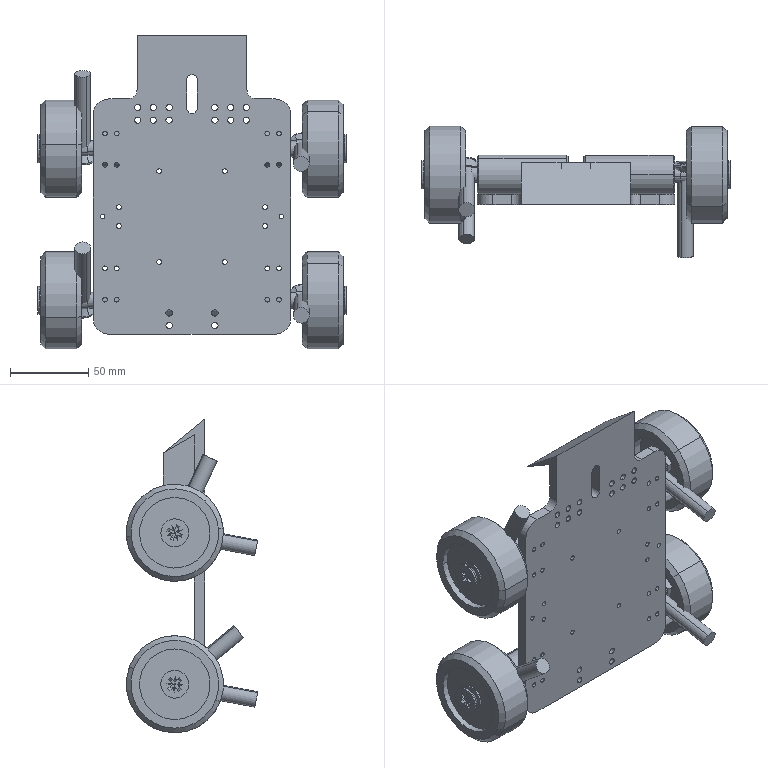Part | SolidWorks | 21 solids | 711 faces | box 196.8 x 83.824 x 200.07 mm | volume 523655 mm3 | plane 378 | cylinder 269 | cone 64 | commonest cylinder face diameters 3 x76 4 x48 0.6 x32 10 x16 17.78 x16 45 x16